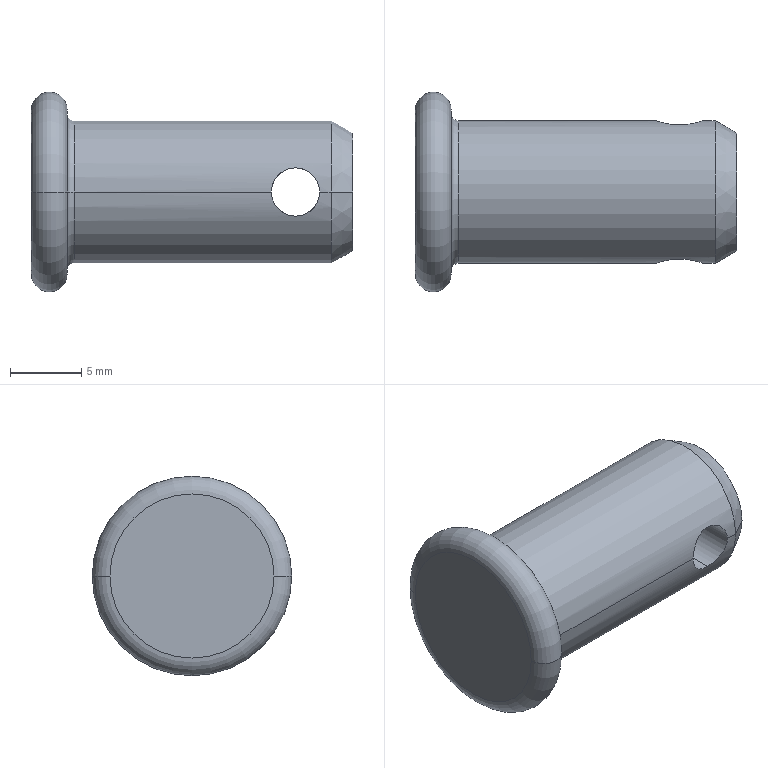Part | SolidWorks | features Cut 1, Fillet 1, Revolution 1 | 1 solid | 13 faces | box 22.5 x 14 x 14 mm | volume 1821 mm3 | cylinder 4 | torus 4 | plane 3 | cone 2 | commonest cylinder face diameters 3.38 x2 10 x2
STEP:
#1=CARTESIAN_POINT('',(18.5,-4.706,-1.69));
#2=VERTEX_POINT('',#1);
#3=CARTESIAN_POINT('',(16.81,-5.,0.));
#4=VERTEX_POINT('',#3);
#5=CARTESIAN_POINT('',(18.5,-4.706,-1.69));
#6=CARTESIAN_POINT('',(18.389,-4.706,-1.69));
#7=CARTESIAN_POINT('',(18.276,-4.71,-1.679));
#8=CARTESIAN_POINT('',(18.059,-4.725,-1.635));
#9=CARTESIAN_POINT('',(17.953,-4.736,-1.603));
#10=CARTESIAN_POINT('',(17.645,-4.779,-1.474));
#11=CARTESIAN_POINT('',(17.46,-4.817,-1.35));
#12=CARTESIAN_POINT('',(17.227,-4.874,-1.116));
#13=CARTESIAN_POINT('',(17.157,-4.893,-1.032));
#14=CARTESIAN_POINT('',(17.035,-4.928,-0.8495));
#15=CARTESIAN_POINT('',(16.982,-4.944,-0.7506));
#16=CARTESIAN_POINT('',(16.855,-4.984,-0.4454));
#17=CARTESIAN_POINT('',(16.81,-5.,-0.2217));
#18=CARTESIAN_POINT('',(16.81,-5.,0.));
#19=B_SPLINE_CURVE_WITH_KNOTS('',3,(#5,#6,#7,#8,#9,#10,#11,#12,#13,#14,#15,#16,#17,#18),.UNSPECIFIED.,.F.,.F.,(4,2,2,2,2,2,4),(0.002662,0.002995,0.003328,0.003993,0.004325,0.004658,0.005323),.UNSPECIFIED.);
#20=EDGE_CURVE('',#2,#4,#19,.T.);
#21=ORIENTED_EDGE('',*,*,#20,.F.);
#22=CARTESIAN_POINT('',(18.5,4.706,-1.69));
#23=VERTEX_POINT('',#22);
#24=CARTESIAN_POINT('',(18.5,-7.,-1.69));
#25=DIRECTION('',(0.,1.,0.));
#26=VECTOR('',#25,1000.);
#27=LINE('',#24,#26);
#28=EDGE_CURVE('',#2,#23,#27,.T.);
#29=ORIENTED_EDGE('',*,*,#28,.T.);
#30=CARTESIAN_POINT('',(16.81,5.,0.));
#31=VERTEX_POINT('',#30);
#32=CARTESIAN_POINT('',(16.81,5.,0.));
#33=CARTESIAN_POINT('',(16.81,5.,-0.1112));
#34=CARTESIAN_POINT('',(16.821,4.996,-0.224));
#35=CARTESIAN_POINT('',(16.865,4.982,-0.4415));
#36=CARTESIAN_POINT('',(16.897,4.971,-0.5472));
#37=CARTESIAN_POINT('',(17.026,4.931,-0.8558));
#38=CARTESIAN_POINT('',(17.15,4.893,-1.041));
#39=CARTESIAN_POINT('',(17.384,4.836,-1.274));
#40=CARTESIAN_POINT('',(17.468,4.817,-1.343));
#41=CARTESIAN_POINT('',(17.651,4.781,-1.465));
#42=CARTESIAN_POINT('',(17.75,4.764,-1.518));
#43=CARTESIAN_POINT('',(17.953,4.736,-1.603));
#44=CARTESIAN_POINT('',(18.058,4.725,-1.635));
#45=CARTESIAN_POINT('',(18.277,4.71,-1.679));
#46=CARTESIAN_POINT('',(18.389,4.706,-1.69));
#47=CARTESIAN_POINT('',(18.5,4.706,-1.69));
#48=B_SPLINE_CURVE_WITH_KNOTS('',3,(#32,#33,#34,#35,#36,#37,#38,#39,#40,#41,#42,#43,#44,#45,#46,#47),.UNSPECIFIED.,.F.,.F.,(4,2,2,2,2,2,2,4),(0.002662,0.002995,0.003328,0.003993,0.004325,0.004658,0.00499,0.005323),.UNSPECIFIED.);
#49=EDGE_CURVE('',#31,#23,#48,.T.);
#50=ORIENTED_EDGE('',*,*,#49,.F.);
#51=CARTESIAN_POINT('',(18.5,4.706,1.69));
#52=VERTEX_POINT('',#51);
#53=CARTESIAN_POINT('',(18.5,4.706,1.69));
#54=CARTESIAN_POINT('',(18.387,4.706,1.69));
#55=CARTESIAN_POINT('',(18.277,4.71,1.679));
#56=CARTESIAN_POINT('',(18.06,4.725,1.635));
#57=CARTESIAN_POINT('',(17.952,4.736,1.602));
#58=CARTESIAN_POINT('',(17.748,4.764,1.517));
#59=CARTESIAN_POINT('',(17.651,4.781,1.465));
#60=CARTESIAN_POINT('',(17.468,4.817,1.343));
#61=CARTESIAN_POINT('',(17.382,4.836,1.272));
#62=CARTESIAN_POINT('',(17.15,4.893,1.04));
#63=CARTESIAN_POINT('',(17.024,4.931,0.8525));
#64=CARTESIAN_POINT('',(16.897,4.971,0.5477));
#65=CARTESIAN_POINT('',(16.865,4.982,0.4402));
#66=CARTESIAN_POINT('',(16.821,4.996,0.2215));
#67=CARTESIAN_POINT('',(16.81,5.,0.1112));
#68=CARTESIAN_POINT('',(16.81,5.,0.));
#69=B_SPLINE_CURVE_WITH_KNOTS('',3,(#53,#54,#55,#56,#57,#58,#59,#60,#61,#62,#63,#64,#65,#66,#67,#68),.UNSPECIFIED.,.F.,.F.,(4,2,2,2,2,2,2,4),(0.,0.0003328,0.0006656,0.0009984,0.001331,0.001997,0.00233,0.002662),.UNSPECIFIED.);
#70=EDGE_CURVE('',#52,#31,#69,.T.);
#71=ORIENTED_EDGE('',*,*,#70,.F.);
#72=CARTESIAN_POINT('',(18.5,-4.706,1.69));
#73=VERTEX_POINT('',#72);
#74=CARTESIAN_POINT('',(18.5,-7.,1.69));
#75=DIRECTION('',(0.,1.,0.));
#76=VECTOR('',#75,1000.);
#77=LINE('',#74,#76);
#78=EDGE_CURVE('',#73,#52,#77,.T.);
#79=ORIENTED_EDGE('',*,*,#78,.F.);
#80=CARTESIAN_POINT('',(16.81,-5.,0.));
#81=CARTESIAN_POINT('',(16.81,-5.,0.2217));
#82=CARTESIAN_POINT('',(16.855,-4.984,0.4454));
#83=CARTESIAN_POINT('',(16.982,-4.944,0.7513));
#84=CARTESIAN_POINT('',(17.035,-4.928,0.8502));
#85=CARTESIAN_POINT('',(17.158,-4.893,1.033));
#86=CARTESIAN_POINT('',(17.227,-4.874,1.117));
#87=CARTESIAN_POINT('',(17.461,-4.817,1.351));
#88=CARTESIAN_POINT('',(17.646,-4.778,1.475));
#89=CARTESIAN_POINT('',(17.953,-4.736,1.603));
#90=CARTESIAN_POINT('',(18.059,-4.725,1.635));
#91=CARTESIAN_POINT('',(18.276,-4.71,1.679));
#92=CARTESIAN_POINT('',(18.389,-4.706,1.69));
#93=CARTESIAN_POINT('',(18.5,-4.706,1.69));
#94=B_SPLINE_CURVE_WITH_KNOTS('',3,(#80,#81,#82,#83,#84,#85,#86,#87,#88,#89,#90,#91,#92,#93),.UNSPECIFIED.,.F.,.F.,(4,2,2,2,2,2,4),(0.005323,0.005988,0.006321,0.006654,0.007319,0.007651,0.007984),.UNSPECIFIED.);
#95=EDGE_CURVE('',#4,#73,#94,.T.);
#96=ORIENTED_EDGE('',*,*,#95,.F.);
#97=EDGE_LOOP('',(#21,#29,#50,#71,#79,#96));
#98=FACE_OUTER_BOUND('',#97,.T.);
#99=CARTESIAN_POINT('',(18.5,-7.,0.));
#100=DIRECTION('',(0.,1.,0.));
#101=DIRECTION('',(0.,0.,1.));
#102=AXIS2_PLACEMENT_3D('',#99,#100,#101);
#103=CYLINDRICAL_SURFACE('',#102,1.69);
#104=ADVANCED_FACE('',(#98),#103,.F.);
#105=CARTESIAN_POINT('',(2.5,5.5,0.));
#106=VERTEX_POINT('',#105);
#107=CARTESIAN_POINT('',(2.5,-5.5,0.));
#108=VERTEX_POINT('',#107);
#109=CARTESIAN_POINT('',(2.5,0.,0.));
#110=DIRECTION('',(-1.,0.,0.));
#111=DIRECTION('',(0.,-1.,0.));
#112=AXIS2_PLACEMENT_3D('',#109,#110,#111);
#113=CIRCLE('',#112,5.5);
#114=EDGE_CURVE('',#106,#108,#113,.T.);
#115=ORIENTED_EDGE('',*,*,#114,.F.);
#116=CARTESIAN_POINT('',(3.,5.,0.));
#117=VERTEX_POINT('',#116);
#118=CARTESIAN_POINT('',(3.,5.5,0.));
#119=DIRECTION('',(0.,0.,1.));
#120=DIRECTION('',(0.,-1.,0.));
#121=AXIS2_PLACEMENT_3D('',#118,#119,#120);
#122=CIRCLE('',#121,0.5);
#123=EDGE_CURVE('',#106,#117,#122,.T.);
#124=ORIENTED_EDGE('',*,*,#123,.T.);
#125=CARTESIAN_POINT('',(3.,-5.,0.));
#126=VERTEX_POINT('',#125);
#127=CARTESIAN_POINT('',(3.,0.,0.));
#128=DIRECTION('',(1.,0.,0.));
#129=DIRECTION('',(0.,-1.,0.));
#130=AXIS2_PLACEMENT_3D('',#127,#128,#129);
#131=CIRCLE('',#130,5.);
#132=EDGE_CURVE('',#126,#117,#131,.T.);
#133=ORIENTED_EDGE('',*,*,#132,.F.);
#134=CARTESIAN_POINT('',(3.,-5.5,0.));
#135=DIRECTION('',(0.,0.,-1.));
#136=DIRECTION('',(-1.,0.,0.));
#137=AXIS2_PLACEMENT_3D('',#134,#135,#136);
#138=CIRCLE('',#137,0.5);
#139=EDGE_CURVE('',#108,#126,#138,.T.);
#140=ORIENTED_EDGE('',*,*,#139,.F.);
#141=EDGE_LOOP('',(#115,#124,#133,#140));
#142=FACE_OUTER_BOUND('',#141,.T.);
#143=CARTESIAN_POINT('',(3.,0.,0.));
#144=DIRECTION('',(-1.,0.,0.));
#145=DIRECTION('',(0.,-1.,0.));
#146=AXIS2_PLACEMENT_3D('',#143,#144,#145);
#147=TOROIDAL_SURFACE('',#146,5.5,0.5);
#148=ADVANCED_FACE('',(#142),#147,.F.);
#149=CARTESIAN_POINT('',(22.5,-4.134,0.));
#150=VERTEX_POINT('',#149);
#151=CARTESIAN_POINT('',(22.5,4.134,0.));
#152=VERTEX_POINT('',#151);
#153=CARTESIAN_POINT('',(22.5,0.,0.));
#154=DIRECTION('',(-1.,0.,0.));
#155=DIRECTION('',(0.,-1.,0.));
#156=AXIS2_PLACEMENT_3D('',#153,#154,#155);
#157=CIRCLE('',#156,4.134);
#158=EDGE_CURVE('',#150,#152,#157,.T.);
#159=ORIENTED_EDGE('',*,*,#158,.T.);
#160=CARTESIAN_POINT('',(21.,5.,0.));
#161=VERTEX_POINT('',#160);
#162=CARTESIAN_POINT('',(22.5,4.134,0.));
#163=DIRECTION('',(-0.866,0.5,0.));
#164=VECTOR('',#163,1000.);
#165=LINE('',#162,#164);
#166=EDGE_CURVE('',#152,#161,#165,.T.);
#167=ORIENTED_EDGE('',*,*,#166,.T.);
#168=CARTESIAN_POINT('',(21.,-5.,0.));
#169=VERTEX_POINT('',#168);
#170=CARTESIAN_POINT('',(21.,0.,0.));
#171=DIRECTION('',(-1.,0.,0.));
#172=DIRECTION('',(0.,-1.,0.));
#173=AXIS2_PLACEMENT_3D('',#170,#171,#172);
#174=CIRCLE('',#173,5.);
#175=EDGE_CURVE('',#169,#161,#174,.T.);
#176=ORIENTED_EDGE('',*,*,#175,.F.);
#177=CARTESIAN_POINT('',(22.5,-4.134,0.));
#178=DIRECTION('',(-0.866,-0.5,0.));
#179=VECTOR('',#178,1000.);
#180=LINE('',#177,#179);
#181=EDGE_CURVE('',#150,#169,#180,.T.);
#182=ORIENTED_EDGE('',*,*,#181,.F.);
#183=EDGE_LOOP('',(#159,#167,#176,#182));
#184=FACE_OUTER_BOUND('',#183,.T.);
#185=CARTESIAN_POINT('',(22.5,0.,0.));
#186=DIRECTION('',(-1.,0.,0.));
#187=DIRECTION('',(0.,-1.,0.));
#188=AXIS2_PLACEMENT_3D('',#185,#186,#187);
#189=CONICAL_SURFACE('',#188,4.134,0.5236);
#190=ADVANCED_FACE('',(#184),#189,.T.);
#191=ORIENTED_EDGE('',*,*,#175,.T.);
#192=CARTESIAN_POINT('',(20.19,5.,0.));
#193=VERTEX_POINT('',#192);
#194=CARTESIAN_POINT('',(-19.83,5.,0.));
#195=DIRECTION('',(-1.,0.,0.));
#196=VECTOR('',#195,1000.);
#197=LINE('',#194,#196);
#198=EDGE_CURVE('',#161,#193,#197,.T.);
#199=ORIENTED_EDGE('',*,*,#198,.T.);
#200=CARTESIAN_POINT('',(20.19,5.,0.));
#201=CARTESIAN_POINT('',(20.19,5.,0.1114));
#202=CARTESIAN_POINT('',(20.179,4.996,0.2217));
#203=CARTESIAN_POINT('',(20.135,4.982,0.4403));
#204=CARTESIAN_POINT('',(20.103,4.971,0.5478));
#205=CARTESIAN_POINT('',(19.975,4.931,0.8532));
#206=CARTESIAN_POINT('',(19.85,4.893,1.04));
#207=CARTESIAN_POINT('',(19.617,4.836,1.273));
#208=CARTESIAN_POINT('',(19.531,4.817,1.343));
#209=CARTESIAN_POINT('',(19.349,4.781,1.466));
#210=CARTESIAN_POINT('',(19.252,4.764,1.517));
#211=CARTESIAN_POINT('',(19.048,4.736,1.603));
#212=CARTESIAN_POINT('',(18.94,4.725,1.635));
#213=CARTESIAN_POINT('',(18.723,4.71,1.679));
#214=CARTESIAN_POINT('',(18.613,4.706,1.69));
#215=CARTESIAN_POINT('',(18.5,4.706,1.69));
#216=B_SPLINE_CURVE_WITH_KNOTS('',3,(#200,#201,#202,#203,#204,#205,#206,#207,#208,#209,#210,#211,#212,#213,#214,#215),.UNSPECIFIED.,.F.,.F.,(4,2,2,2,2,2,2,4),(0.007984,0.008316,0.008649,0.009314,0.009647,0.009979,0.01031,0.01064),.UNSPECIFIED.);
#217=EDGE_CURVE('',#193,#52,#216,.T.);
#218=ORIENTED_EDGE('',*,*,#217,.T.);
#219=ORIENTED_EDGE('',*,*,#70,.T.);
#220=CARTESIAN_POINT('',(-19.83,5.,0.));
#221=DIRECTION('',(-1.,0.,0.));
#222=VECTOR('',#221,1000.);
#223=LINE('',#220,#222);
#224=EDGE_CURVE('',#31,#117,#223,.T.);
#225=ORIENTED_EDGE('',*,*,#224,.T.);
#226=CARTESIAN_POINT('',(3.,0.,0.));
#227=DIRECTION('',(1.,0.,0.));
#228=DIRECTION('',(0.,-1.,0.));
#229=AXIS2_PLACEMENT_3D('',#226,#227,#228);
#230=CIRCLE('',#229,5.);
#231=EDGE_CURVE('',#117,#126,#230,.T.);
#232=ORIENTED_EDGE('',*,*,#231,.T.);
#233=CARTESIAN_POINT('',(-19.83,-5.,0.));
#234=DIRECTION('',(-1.,0.,0.));
#235=VECTOR('',#234,1000.);
#236=LINE('',#233,#235);
#237=EDGE_CURVE('',#4,#126,#236,.T.);
#238=ORIENTED_EDGE('',*,*,#237,.F.);
#239=ORIENTED_EDGE('',*,*,#95,.T.);
#240=CARTESIAN_POINT('',(20.19,-5.,0.));
#241=VERTEX_POINT('',#240);
#242=CARTESIAN_POINT('',(18.5,-4.706,1.69));
#243=CARTESIAN_POINT('',(18.611,-4.706,1.69));
#244=CARTESIAN_POINT('',(18.722,-4.71,1.679));
#245=CARTESIAN_POINT('',(18.94,-4.725,1.635));
#246=CARTESIAN_POINT('',(19.048,-4.736,1.603));
#247=CARTESIAN_POINT('',(19.353,-4.778,1.476));
#248=CARTESIAN_POINT('',(19.54,-4.817,1.35));
#249=CARTESIAN_POINT('',(19.772,-4.874,1.118));
#250=CARTESIAN_POINT('',(19.843,-4.893,1.032));
#251=CARTESIAN_POINT('',(19.965,-4.928,0.8489));
#252=CARTESIAN_POINT('',(20.017,-4.944,0.7523));
#253=CARTESIAN_POINT('',(20.103,-4.971,0.5479));
#254=CARTESIAN_POINT('',(20.135,-4.982,0.4401));
#255=CARTESIAN_POINT('',(20.179,-4.996,0.2231));
#256=CARTESIAN_POINT('',(20.19,-5.,0.1125));
#257=CARTESIAN_POINT('',(20.19,-5.,0.));
#258=B_SPLINE_CURVE_WITH_KNOTS('',3,(#242,#243,#244,#245,#246,#247,#248,#249,#250,#251,#252,#253,#254,#255,#256,#257),.UNSPECIFIED.,.F.,.F.,(4,2,2,2,2,2,2,4),(0.007984,0.008317,0.008649,0.009314,0.009647,0.00998,0.01031,0.01065),.UNSPECIFIED.);
#259=EDGE_CURVE('',#73,#241,#258,.T.);
#260=ORIENTED_EDGE('',*,*,#259,.T.);
#261=CARTESIAN_POINT('',(-19.83,-5.,0.));
#262=DIRECTION('',(-1.,0.,0.));
#263=VECTOR('',#262,1000.);
#264=LINE('',#261,#263);
#265=EDGE_CURVE('',#169,#241,#264,.T.);
#266=ORIENTED_EDGE('',*,*,#265,.F.);
#267=EDGE_LOOP('',(#191,#199,#218,#219,#225,#232,#238,#239,#260,#266));
#268=FACE_OUTER_BOUND('',#267,.T.);
#269=CARTESIAN_POINT('',(-19.83,0.,0.));
#270=DIRECTION('',(-1.,0.,0.));
#271=DIRECTION('',(0.,-1.,0.));
#272=AXIS2_PLACEMENT_3D('',#269,#270,#271);
#273=CYLINDRICAL_SURFACE('',#272,5.);
#274=ADVANCED_FACE('',(#268),#273,.T.);
#275=CARTESIAN_POINT('',(2.5,-5.75,0.));
#276=VERTEX_POINT('',#275);
#277=CARTESIAN_POINT('',(2.5,5.75,0.));
#278=VERTEX_POINT('',#277);
#279=CARTESIAN_POINT('',(2.5,0.,0.));
#280=DIRECTION('',(-1.,0.,0.));
#281=DIRECTION('',(0.,-1.,0.));
#282=AXIS2_PLACEMENT_3D('',#279,#280,#281);
#283=CIRCLE('',#282,5.75);
#284=EDGE_CURVE('',#276,#278,#283,.T.);
#285=ORIENTED_EDGE('',*,*,#284,.T.);
#286=CARTESIAN_POINT('',(0.,5.75,0.));
#287=VERTEX_POINT('',#286);
#288=CARTESIAN_POINT('',(1.25,5.75,0.));
#289=DIRECTION('',(0.,0.,1.));
#290=DIRECTION('',(0.,-1.,0.));
#291=AXIS2_PLACEMENT_3D('',#288,#289,#290);
#292=CIRCLE('',#291,1.25);
#293=EDGE_CURVE('',#278,#287,#292,.T.);
#294=ORIENTED_EDGE('',*,*,#293,.T.);
#295=CARTESIAN_POINT('',(0.,-5.75,0.));
#296=VERTEX_POINT('',#295);
#297=CARTESIAN_POINT('',(0.,0.,0.));
#298=DIRECTION('',(-1.,0.,0.));
#299=DIRECTION('',(0.,-1.,0.));
#300=AXIS2_PLACEMENT_3D('',#297,#298,#299);
#301=CIRCLE('',#300,5.75);
#302=EDGE_CURVE('',#296,#287,#301,.T.);
#303=ORIENTED_EDGE('',*,*,#302,.F.);
#304=CARTESIAN_POINT('',(1.25,-5.75,0.));
#305=DIRECTION('',(0.,0.,-1.));
#306=DIRECTION('',(-1.,0.,0.));
#307=AXIS2_PLACEMENT_3D('',#304,#305,#306);
#308=CIRCLE('',#307,1.25);
#309=EDGE_CURVE('',#276,#296,#308,.T.);
#310=ORIENTED_EDGE('',*,*,#309,.F.);
#311=EDGE_LOOP('',(#285,#294,#303,#310));
#312=FACE_OUTER_BOUND('',#311,.T.);
#313=CARTESIAN_POINT('',(1.25,0.,0.));
#314=DIRECTION('',(-1.,0.,0.));
#315=DIRECTION('',(0.,-1.,0.));
#316=AXIS2_PLACEMENT_3D('',#313,#314,#315);
#317=TOROIDAL_SURFACE('',#316,5.75,1.25);
#318=ADVANCED_FACE('',(#312),#317,.T.);
#319=ORIENTED_EDGE('',*,*,#158,.F.);
#320=CARTESIAN_POINT('',(22.5,0.,0.));
#321=DIRECTION('',(-1.,0.,0.));
#322=DIRECTION('',(0.,-1.,0.));
#323=AXIS2_PLACEMENT_3D('',#320,#321,#322);
#324=CIRCLE('',#323,4.134);
#325=EDGE_CURVE('',#152,#150,#324,.T.);
#326=ORIENTED_EDGE('',*,*,#325,.F.);
#327=EDGE_LOOP('',(#319,#326));
#328=FACE_OUTER_BOUND('',#327,.T.);
#329=CARTESIAN_POINT('',(22.5,0.,0.));
#330=DIRECTION('',(-1.,0.,0.));
#331=DIRECTION('',(0.,-1.,0.));
#332=AXIS2_PLACEMENT_3D('',#329,#330,#331);
#333=PLANE('',#332);
#334=ADVANCED_FACE('',(#328),#333,.F.);
#335=ORIENTED_EDGE('',*,*,#302,.T.);
#336=CARTESIAN_POINT('',(0.,0.,0.));
#337=DIRECTION('',(-1.,0.,0.));
#338=DIRECTION('',(0.,-1.,0.));
#339=AXIS2_PLACEMENT_3D('',#336,#337,#338);
#340=CIRCLE('',#339,5.75);
#341=EDGE_CURVE('',#287,#296,#340,.T.);
#342=ORIENTED_EDGE('',*,*,#341,.T.);
#343=EDGE_LOOP('',(#335,#342));
#344=FACE_OUTER_BOUND('',#343,.T.);
#345=CARTESIAN_POINT('',(0.,0.,0.));
#346=DIRECTION('',(1.,0.,0.));
#347=DIRECTION('',(0.,1.,0.));
#348=AXIS2_PLACEMENT_3D('',#345,#346,#347);
#349=PLANE('',#348);
#350=ADVANCED_FACE('',(#344),#349,.F.);
#351=ORIENTED_EDGE('',*,*,#293,.F.);
#352=CARTESIAN_POINT('',(2.5,0.,0.));
#353=DIRECTION('',(-1.,0.,0.));
#354=DIRECTION('',(0.,-1.,0.));
#355=AXIS2_PLACEMENT_3D('',#352,#353,#354);
#356=CIRCLE('',#355,5.75);
#357=EDGE_CURVE('',#278,#276,#356,.T.);
#358=ORIENTED_EDGE('',*,*,#357,.T.);
#359=ORIENTED_EDGE('',*,*,#309,.T.);
#360=ORIENTED_EDGE('',*,*,#341,.F.);
#361=EDGE_LOOP('',(#351,#358,#359,#360));
#362=FACE_OUTER_BOUND('',#361,.T.);
#363=CARTESIAN_POINT('',(1.25,0.,0.));
#364=DIRECTION('',(-1.,0.,0.));
#365=DIRECTION('',(0.,-1.,0.));
#366=AXIS2_PLACEMENT_3D('',#363,#364,#365);
#367=TOROIDAL_SURFACE('',#366,5.75,1.25);
#368=ADVANCED_FACE('',(#362),#367,.T.);
#369=CARTESIAN_POINT('',(2.5,0.,0.));
#370=DIRECTION('',(-1.,0.,0.));
#371=DIRECTION('',(0.,-1.,0.));
#372=AXIS2_PLACEMENT_3D('',#369,#370,#371);
#373=CIRCLE('',#372,5.5);
#374=EDGE_CURVE('',#108,#106,#373,.T.);
#375=ORIENTED_EDGE('',*,*,#374,.T.);
#376=ORIENTED_EDGE('',*,*,#114,.T.);
#377=EDGE_LOOP('',(#375,#376));
#378=FACE_BOUND('',#377,.T.);
#379=ORIENTED_EDGE('',*,*,#284,.F.);
#380=ORIENTED_EDGE('',*,*,#357,.F.);
#381=EDGE_LOOP('',(#379,#380));
#382=FACE_OUTER_BOUND('',#381,.T.);
#383=CARTESIAN_POINT('',(2.5,5.,0.));
#384=DIRECTION('',(-1.,0.,0.));
#385=DIRECTION('',(0.,-1.,0.));
#386=AXIS2_PLACEMENT_3D('',#383,#384,#385);
#387=PLANE('',#386);
#388=ADVANCED_FACE('',(#378,#382),#387,.F.);
#389=ORIENTED_EDGE('',*,*,#198,.F.);
#390=CARTESIAN_POINT('',(21.,0.,0.));
#391=DIRECTION('',(-1.,0.,0.));
#392=DIRECTION('',(0.,-1.,0.));
#393=AXIS2_PLACEMENT_3D('',#390,#391,#392);
#394=CIRCLE('',#393,5.);
#395=EDGE_CURVE('',#161,#169,#394,.T.);
#396=ORIENTED_EDGE('',*,*,#395,.T.);
#397=ORIENTED_EDGE('',*,*,#265,.T.);
#398=CARTESIAN_POINT('',(20.19,-5.,0.));
#399=CARTESIAN_POINT('',(20.19,-5.,-0.1126));
#400=CARTESIAN_POINT('',(20.179,-4.996,-0.2231));
#401=CARTESIAN_POINT('',(20.135,-4.982,-0.4404));
#402=CARTESIAN_POINT('',(20.102,-4.971,-0.5482));
#403=CARTESIAN_POINT('',(20.017,-4.944,-0.7526));
#404=CARTESIAN_POINT('',(19.965,-4.928,-0.8494));
#405=CARTESIAN_POINT('',(19.842,-4.893,-1.033));
#406=CARTESIAN_POINT('',(19.772,-4.874,-1.119));
#407=CARTESIAN_POINT('',(19.539,-4.817,-1.35));
#408=CARTESIAN_POINT('',(19.352,-4.778,-1.476));
#409=CARTESIAN_POINT('',(19.048,-4.736,-1.603));
#410=CARTESIAN_POINT('',(18.94,-4.725,-1.635));
#411=CARTESIAN_POINT('',(18.721,-4.71,-1.679));
#412=CARTESIAN_POINT('',(18.611,-4.706,-1.69));
#413=CARTESIAN_POINT('',(18.5,-4.706,-1.69));
#414=B_SPLINE_CURVE_WITH_KNOTS('',3,(#398,#399,#400,#401,#402,#403,#404,#405,#406,#407,#408,#409,#410,#411,#412,#413),.UNSPECIFIED.,.F.,.F.,(4,2,2,2,2,2,2,4),(0.,0.0003328,0.0006656,0.0009984,0.001331,0.001997,0.00233,0.002662),.UNSPECIFIED.);
#415=EDGE_CURVE('',#241,#2,#414,.T.);
#416=ORIENTED_EDGE('',*,*,#415,.T.);
#417=ORIENTED_EDGE('',*,*,#20,.T.);
#418=ORIENTED_EDGE('',*,*,#237,.T.);
#419=ORIENTED_EDGE('',*,*,#132,.T.);
#420=ORIENTED_EDGE('',*,*,#224,.F.);
#421=ORIENTED_EDGE('',*,*,#49,.T.);
#422=CARTESIAN_POINT('',(18.5,4.706,-1.69));
#423=CARTESIAN_POINT('',(18.722,4.706,-1.69));
#424=CARTESIAN_POINT('',(18.945,4.722,-1.645));
#425=CARTESIAN_POINT('',(19.251,4.764,-1.518));
#426=CARTESIAN_POINT('',(19.35,4.781,-1.465));
#427=CARTESIAN_POINT('',(19.532,4.817,-1.343));
#428=CARTESIAN_POINT('',(19.617,4.836,-1.273));
#429=CARTESIAN_POINT('',(19.851,4.893,-1.039));
#430=CARTESIAN_POINT('',(19.975,4.931,-0.8548));
#431=CARTESIAN_POINT('',(20.103,4.971,-0.5467));
#432=CARTESIAN_POINT('',(20.135,4.982,-0.4411));
#433=CARTESIAN_POINT('',(20.179,4.996,-0.2241));
#434=CARTESIAN_POINT('',(20.19,5.,-0.1113));
#435=CARTESIAN_POINT('',(20.19,5.,0.));
#436=B_SPLINE_CURVE_WITH_KNOTS('',3,(#422,#423,#424,#425,#426,#427,#428,#429,#430,#431,#432,#433,#434,#435),.UNSPECIFIED.,.F.,.F.,(4,2,2,2,2,2,4),(0.005323,0.005988,0.006321,0.006653,0.007318,0.007651,0.007984),.UNSPECIFIED.);
#437=EDGE_CURVE('',#23,#193,#436,.T.);
#438=ORIENTED_EDGE('',*,*,#437,.T.);
#439=EDGE_LOOP('',(#389,#396,#397,#416,#417,#418,#419,#420,#421,#438));
#440=FACE_OUTER_BOUND('',#439,.T.);
#441=CARTESIAN_POINT('',(-19.83,0.,0.));
#442=DIRECTION('',(-1.,0.,0.));
#443=DIRECTION('',(0.,-1.,0.));
#444=AXIS2_PLACEMENT_3D('',#441,#442,#443);
#445=CYLINDRICAL_SURFACE('',#444,5.);
#446=ADVANCED_FACE('',(#440),#445,.T.);
#447=ORIENTED_EDGE('',*,*,#166,.F.);
#448=ORIENTED_EDGE('',*,*,#325,.T.);
#449=ORIENTED_EDGE('',*,*,#181,.T.);
#450=ORIENTED_EDGE('',*,*,#395,.F.);
#451=EDGE_LOOP('',(#447,#448,#449,#450));
#452=FACE_OUTER_BOUND('',#451,.T.);
#453=CARTESIAN_POINT('',(22.5,0.,0.));
#454=DIRECTION('',(-1.,0.,0.));
#455=DIRECTION('',(0.,-1.,0.));
#456=AXIS2_PLACEMENT_3D('',#453,#454,#455);
#457=CONICAL_SURFACE('',#456,4.134,0.5236);
#458=ADVANCED_FACE('',(#452),#457,.T.);
#459=ORIENTED_EDGE('',*,*,#123,.F.);
#460=ORIENTED_EDGE('',*,*,#374,.F.);
#461=ORIENTED_EDGE('',*,*,#139,.T.);
#462=ORIENTED_EDGE('',*,*,#231,.F.);
#463=EDGE_LOOP('',(#459,#460,#461,#462));
#464=FACE_OUTER_BOUND('',#463,.T.);
#465=CARTESIAN_POINT('',(3.,0.,0.));
#466=DIRECTION('',(-1.,0.,0.));
#467=DIRECTION('',(0.,-1.,0.));
#468=AXIS2_PLACEMENT_3D('',#465,#466,#467);
#469=TOROIDAL_SURFACE('',#468,5.5,0.5);
#470=ADVANCED_FACE('',(#464),#469,.F.);
#471=ORIENTED_EDGE('',*,*,#28,.F.);
#472=ORIENTED_EDGE('',*,*,#415,.F.);
#473=ORIENTED_EDGE('',*,*,#259,.F.);
#474=ORIENTED_EDGE('',*,*,#78,.T.);
#475=ORIENTED_EDGE('',*,*,#217,.F.);
#476=ORIENTED_EDGE('',*,*,#437,.F.);
#477=EDGE_LOOP('',(#471,#472,#473,#474,#475,#476));
#478=FACE_OUTER_BOUND('',#477,.T.);
#479=CARTESIAN_POINT('',(18.5,-7.,0.));
#480=DIRECTION('',(0.,1.,0.));
#481=DIRECTION('',(0.,0.,1.));
#482=AXIS2_PLACEMENT_3D('',#479,#480,#481);
#483=CYLINDRICAL_SURFACE('',#482,1.69);
#484=ADVANCED_FACE('',(#478),#483,.F.);
#485=CLOSED_SHELL('',(#104,#148,#190,#274,#318,#334,#350,#368,#388,#446,#458,#470,#484));
#486=MANIFOLD_SOLID_BREP('',#485);
#487=CARTESIAN_POINT('',(0.,0.,0.));
#488=DIRECTION('',(0.,0.,1.));
#489=DIRECTION('',(1.,0.,0.));
#490=AXIS2_PLACEMENT_3D('',#487,#488,#489);
#491=(LENGTH_UNIT()NAMED_UNIT(*)SI_UNIT(.MILLI.,.METRE.));
#492=UNCERTAINTY_MEASURE_WITH_UNIT(LENGTH_MEASURE(0.00001),#491,'','');
#493=(NAMED_UNIT(*)PLANE_ANGLE_UNIT()SI_UNIT($,.RADIAN.));
#494=(NAMED_UNIT(*)SI_UNIT($,.STERADIAN.)SOLID_ANGLE_UNIT());
#495=(GEOMETRIC_REPRESENTATION_CONTEXT(3)GLOBAL_UNCERTAINTY_ASSIGNED_CONTEXT((#492))GLOBAL_UNIT_ASSIGNED_CONTEXT((#491,#493,#494))REPRESENTATION_CONTEXT('',''));
#496=ADVANCED_BREP_SHAPE_REPRESENTATION('',(#486,#490),#495);